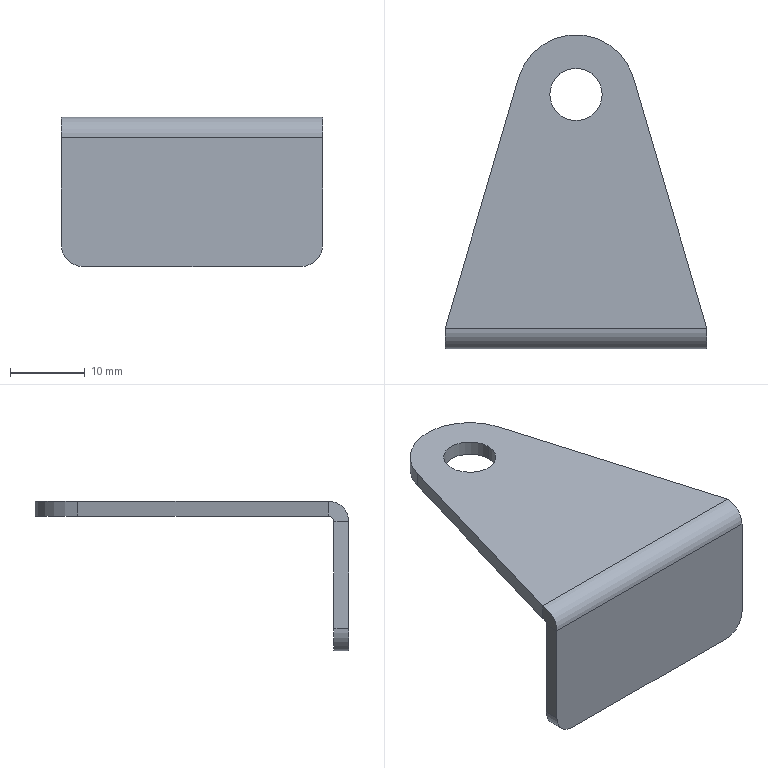Part | SolidWorks | features ICE 2, EdgeFlange 1, Fillet 1, FlatPattern 1, HoleWzd 1, SMBaseFlange 1, SheetMetal 1 | 1 solid | 18 faces | box 35 x 42 x 20 mm | volume 3132 mm3 | plane 11 | cylinder 7 | commonest cylinder face diameters 6 x2 7 x2 1.473 x1 5.473 x1 16 x1
STEP:
#1=CARTESIAN_POINT('',(3.5,32.,8.));
#2=VERTEX_POINT('',#1);
#3=CARTESIAN_POINT('',(-3.5,32.,8.));
#4=VERTEX_POINT('',#3);
#5=CARTESIAN_POINT('',(0.,32.,8.));
#6=DIRECTION('',(0.,0.,-1.));
#7=DIRECTION('',(-1.,0.,0.));
#8=AXIS2_PLACEMENT_3D('',#5,#6,#7);
#9=CIRCLE('',#8,3.5);
#10=EDGE_CURVE('',#2,#4,#9,.T.);
#11=ORIENTED_EDGE('',*,*,#10,.T.);
#12=CARTESIAN_POINT('',(-3.5,32.,10.));
#13=VERTEX_POINT('',#12);
#14=CARTESIAN_POINT('',(-3.5,32.,10.));
#15=DIRECTION('',(0.,0.,1.));
#16=VECTOR('',#15,1000.);
#17=LINE('',#14,#16);
#18=EDGE_CURVE('',#4,#13,#17,.T.);
#19=ORIENTED_EDGE('',*,*,#18,.T.);
#20=CARTESIAN_POINT('',(3.5,32.,10.));
#21=VERTEX_POINT('',#20);
#22=CARTESIAN_POINT('',(0.,32.,10.));
#23=DIRECTION('',(0.,0.,1.));
#24=DIRECTION('',(1.,0.,0.));
#25=AXIS2_PLACEMENT_3D('',#22,#23,#24);
#26=CIRCLE('',#25,3.5);
#27=EDGE_CURVE('',#13,#21,#26,.T.);
#28=ORIENTED_EDGE('',*,*,#27,.T.);
#29=CARTESIAN_POINT('',(3.5,32.,10.));
#30=DIRECTION('',(0.,0.,1.));
#31=VECTOR('',#30,1000.);
#32=LINE('',#29,#31);
#33=EDGE_CURVE('',#2,#21,#32,.T.);
#34=ORIENTED_EDGE('',*,*,#33,.F.);
#35=EDGE_LOOP('',(#11,#19,#28,#34));
#36=FACE_OUTER_BOUND('',#35,.T.);
#37=CARTESIAN_POINT('',(0.,32.,10.));
#38=DIRECTION('',(0.,0.,1.));
#39=DIRECTION('',(1.,0.,0.));
#40=AXIS2_PLACEMENT_3D('',#37,#38,#39);
#41=CYLINDRICAL_SURFACE('',#40,3.5);
#42=ADVANCED_FACE('',(#36),#41,.F.);
#43=CARTESIAN_POINT('',(0.,32.,10.));
#44=DIRECTION('',(0.,0.,1.));
#45=DIRECTION('',(1.,0.,0.));
#46=AXIS2_PLACEMENT_3D('',#43,#44,#45);
#47=CIRCLE('',#46,3.5);
#48=EDGE_CURVE('',#21,#13,#47,.T.);
#49=ORIENTED_EDGE('',*,*,#48,.F.);
#50=ORIENTED_EDGE('',*,*,#27,.F.);
#51=EDGE_LOOP('',(#49,#50));
#52=FACE_BOUND('',#51,.T.);
#53=CARTESIAN_POINT('',(-7.677,34.25,10.));
#54=VERTEX_POINT('',#53);
#55=CARTESIAN_POINT('',(7.677,34.25,10.));
#56=VERTEX_POINT('',#55);
#57=CARTESIAN_POINT('',(0.,32.,10.));
#58=DIRECTION('',(0.,0.,-1.));
#59=DIRECTION('',(-1.,0.,0.));
#60=AXIS2_PLACEMENT_3D('',#57,#58,#59);
#61=CIRCLE('',#60,8.);
#62=EDGE_CURVE('',#54,#56,#61,.T.);
#63=ORIENTED_EDGE('',*,*,#62,.F.);
#64=CARTESIAN_POINT('',(-17.5,0.7366,10.));
#65=VERTEX_POINT('',#64);
#66=CARTESIAN_POINT('',(-16.314,4.782,10.));
#67=DIRECTION('',(0.2813,0.9596,0.));
#68=VECTOR('',#67,1000.);
#69=LINE('',#66,#68);
#70=EDGE_CURVE('',#65,#54,#69,.T.);
#71=ORIENTED_EDGE('',*,*,#70,.F.);
#72=CARTESIAN_POINT('',(17.5,0.7366,10.));
#73=VERTEX_POINT('',#72);
#74=CARTESIAN_POINT('',(-17.5,0.7366,10.));
#75=DIRECTION('',(-1.,0.,0.));
#76=VECTOR('',#75,1000.);
#77=LINE('',#74,#76);
#78=EDGE_CURVE('',#73,#65,#77,.T.);
#79=ORIENTED_EDGE('',*,*,#78,.F.);
#80=CARTESIAN_POINT('',(16.314,4.782,10.));
#81=DIRECTION('',(0.2813,-0.9596,0.));
#82=VECTOR('',#81,1000.);
#83=LINE('',#80,#82);
#84=EDGE_CURVE('',#56,#73,#83,.T.);
#85=ORIENTED_EDGE('',*,*,#84,.F.);
#86=EDGE_LOOP('',(#63,#71,#79,#85));
#87=FACE_OUTER_BOUND('',#86,.T.);
#88=CARTESIAN_POINT('',(0.,0.,10.));
#89=DIRECTION('',(0.,0.,-1.));
#90=DIRECTION('',(-1.,0.,0.));
#91=AXIS2_PLACEMENT_3D('',#88,#89,#90);
#92=PLANE('',#91);
#93=ADVANCED_FACE('',(#52,#87),#92,.F.);
#94=ORIENTED_EDGE('',*,*,#10,.F.);
#95=CARTESIAN_POINT('',(0.,32.,8.));
#96=DIRECTION('',(0.,0.,-1.));
#97=DIRECTION('',(-1.,0.,0.));
#98=AXIS2_PLACEMENT_3D('',#95,#96,#97);
#99=CIRCLE('',#98,3.5);
#100=EDGE_CURVE('',#4,#2,#99,.T.);
#101=ORIENTED_EDGE('',*,*,#100,.F.);
#102=EDGE_LOOP('',(#94,#101));
#103=FACE_BOUND('',#102,.T.);
#104=CARTESIAN_POINT('',(-17.5,0.7366,8.));
#105=VERTEX_POINT('',#104);
#106=CARTESIAN_POINT('',(-7.677,34.25,8.));
#107=VERTEX_POINT('',#106);
#108=CARTESIAN_POINT('',(-16.314,4.782,8.));
#109=DIRECTION('',(0.2813,0.9596,0.));
#110=VECTOR('',#109,1000.);
#111=LINE('',#108,#110);
#112=EDGE_CURVE('',#105,#107,#111,.T.);
#113=ORIENTED_EDGE('',*,*,#112,.T.);
#114=CARTESIAN_POINT('',(7.677,34.25,8.));
#115=VERTEX_POINT('',#114);
#116=CARTESIAN_POINT('',(0.,32.,8.));
#117=DIRECTION('',(0.,0.,-1.));
#118=DIRECTION('',(-1.,0.,0.));
#119=AXIS2_PLACEMENT_3D('',#116,#117,#118);
#120=CIRCLE('',#119,8.);
#121=EDGE_CURVE('',#107,#115,#120,.T.);
#122=ORIENTED_EDGE('',*,*,#121,.T.);
#123=CARTESIAN_POINT('',(17.5,0.7366,8.));
#124=VERTEX_POINT('',#123);
#125=CARTESIAN_POINT('',(16.314,4.782,8.));
#126=DIRECTION('',(0.2813,-0.9596,0.));
#127=VECTOR('',#126,1000.);
#128=LINE('',#125,#127);
#129=EDGE_CURVE('',#115,#124,#128,.T.);
#130=ORIENTED_EDGE('',*,*,#129,.T.);
#131=CARTESIAN_POINT('',(-17.5,0.7366,8.));
#132=DIRECTION('',(1.,0.,0.));
#133=VECTOR('',#132,1000.);
#134=LINE('',#131,#133);
#135=EDGE_CURVE('',#105,#124,#134,.T.);
#136=ORIENTED_EDGE('',*,*,#135,.F.);
#137=EDGE_LOOP('',(#113,#122,#130,#136));
#138=FACE_OUTER_BOUND('',#137,.T.);
#139=CARTESIAN_POINT('',(0.,0.,8.));
#140=DIRECTION('',(0.,0.,-1.));
#141=DIRECTION('',(-1.,0.,0.));
#142=AXIS2_PLACEMENT_3D('',#139,#140,#141);
#143=PLANE('',#142);
#144=ADVANCED_FACE('',(#103,#138),#143,.T.);
#145=CARTESIAN_POINT('',(17.5,-2.,7.263));
#146=VERTEX_POINT('',#145);
#147=CARTESIAN_POINT('',(17.5,-2.,-7.));
#148=VERTEX_POINT('',#147);
#149=CARTESIAN_POINT('',(17.5,-2.,10.));
#150=DIRECTION('',(0.,0.,-1.));
#151=VECTOR('',#150,1000.);
#152=LINE('',#149,#151);
#153=EDGE_CURVE('',#146,#148,#152,.T.);
#154=ORIENTED_EDGE('',*,*,#153,.T.);
#155=CARTESIAN_POINT('',(17.5,0.,-7.));
#156=VERTEX_POINT('',#155);
#157=CARTESIAN_POINT('',(17.5,-2.,-7.));
#158=DIRECTION('',(0.,1.,0.));
#159=VECTOR('',#158,1000.);
#160=LINE('',#157,#159);
#161=EDGE_CURVE('',#148,#156,#160,.T.);
#162=ORIENTED_EDGE('',*,*,#161,.T.);
#163=CARTESIAN_POINT('',(17.5,0.,7.263));
#164=VERTEX_POINT('',#163);
#165=CARTESIAN_POINT('',(17.5,0.,10.));
#166=DIRECTION('',(0.,0.,-1.));
#167=VECTOR('',#166,1000.);
#168=LINE('',#165,#167);
#169=EDGE_CURVE('',#164,#156,#168,.T.);
#170=ORIENTED_EDGE('',*,*,#169,.F.);
#171=CARTESIAN_POINT('',(17.5,0.,7.263));
#172=DIRECTION('',(0.,-1.,0.));
#173=VECTOR('',#172,1000.);
#174=LINE('',#171,#173);
#175=EDGE_CURVE('',#164,#146,#174,.T.);
#176=ORIENTED_EDGE('',*,*,#175,.T.);
#177=EDGE_LOOP('',(#154,#162,#170,#176));
#178=FACE_OUTER_BOUND('',#177,.T.);
#179=CARTESIAN_POINT('',(17.5,-2.,10.));
#180=DIRECTION('',(1.,0.,0.));
#181=DIRECTION('',(0.,0.,-1.));
#182=AXIS2_PLACEMENT_3D('',#179,#180,#181);
#183=PLANE('',#182);
#184=ADVANCED_FACE('',(#178),#183,.T.);
#185=CARTESIAN_POINT('',(14.5,-2.,-10.));
#186=VERTEX_POINT('',#185);
#187=CARTESIAN_POINT('',(-14.5,-2.,-10.));
#188=VERTEX_POINT('',#187);
#189=CARTESIAN_POINT('',(-17.5,-2.,-10.));
#190=DIRECTION('',(-1.,0.,0.));
#191=VECTOR('',#190,1000.);
#192=LINE('',#189,#191);
#193=EDGE_CURVE('',#186,#188,#192,.T.);
#194=ORIENTED_EDGE('',*,*,#193,.F.);
#195=CARTESIAN_POINT('',(14.5,-2.,-7.));
#196=DIRECTION('',(0.,-1.,0.));
#197=DIRECTION('',(0.,0.,-1.));
#198=AXIS2_PLACEMENT_3D('',#195,#196,#197);
#199=CIRCLE('',#198,3.);
#200=EDGE_CURVE('',#186,#148,#199,.T.);
#201=ORIENTED_EDGE('',*,*,#200,.T.);
#202=ORIENTED_EDGE('',*,*,#153,.F.);
#203=CARTESIAN_POINT('',(-17.5,-2.,7.263));
#204=VERTEX_POINT('',#203);
#205=CARTESIAN_POINT('',(17.5,-2.,7.263));
#206=DIRECTION('',(-1.,0.,0.));
#207=VECTOR('',#206,1000.);
#208=LINE('',#205,#207);
#209=EDGE_CURVE('',#146,#204,#208,.T.);
#210=ORIENTED_EDGE('',*,*,#209,.T.);
#211=CARTESIAN_POINT('',(-17.5,-2.,-7.));
#212=VERTEX_POINT('',#211);
#213=CARTESIAN_POINT('',(-17.5,-2.,10.));
#214=DIRECTION('',(0.,0.,1.));
#215=VECTOR('',#214,1000.);
#216=LINE('',#213,#215);
#217=EDGE_CURVE('',#212,#204,#216,.T.);
#218=ORIENTED_EDGE('',*,*,#217,.F.);
#219=CARTESIAN_POINT('',(-14.5,-2.,-7.));
#220=DIRECTION('',(0.,-1.,0.));
#221=DIRECTION('',(0.,0.,-1.));
#222=AXIS2_PLACEMENT_3D('',#219,#220,#221);
#223=CIRCLE('',#222,3.);
#224=EDGE_CURVE('',#212,#188,#223,.T.);
#225=ORIENTED_EDGE('',*,*,#224,.T.);
#226=EDGE_LOOP('',(#194,#201,#202,#210,#218,#225));
#227=FACE_OUTER_BOUND('',#226,.T.);
#228=CARTESIAN_POINT('',(0.,-2.,0.));
#229=DIRECTION('',(0.,-1.,0.));
#230=DIRECTION('',(0.,0.,-1.));
#231=AXIS2_PLACEMENT_3D('',#228,#229,#230);
#232=PLANE('',#231);
#233=ADVANCED_FACE('',(#227),#232,.T.);
#234=ORIENTED_EDGE('',*,*,#169,.T.);
#235=CARTESIAN_POINT('',(14.5,0.,-10.));
#236=VERTEX_POINT('',#235);
#237=CARTESIAN_POINT('',(14.5,0.,-7.));
#238=DIRECTION('',(0.,1.,0.));
#239=DIRECTION('',(0.,0.,-1.));
#240=AXIS2_PLACEMENT_3D('',#237,#238,#239);
#241=CIRCLE('',#240,3.);
#242=EDGE_CURVE('',#156,#236,#241,.T.);
#243=ORIENTED_EDGE('',*,*,#242,.T.);
#244=CARTESIAN_POINT('',(-14.5,0.,-10.));
#245=VERTEX_POINT('',#244);
#246=CARTESIAN_POINT('',(-17.5,0.,-10.));
#247=DIRECTION('',(-1.,0.,0.));
#248=VECTOR('',#247,1000.);
#249=LINE('',#246,#248);
#250=EDGE_CURVE('',#236,#245,#249,.T.);
#251=ORIENTED_EDGE('',*,*,#250,.T.);
#252=CARTESIAN_POINT('',(-17.5,0.,-7.));
#253=VERTEX_POINT('',#252);
#254=CARTESIAN_POINT('',(-14.5,0.,-7.));
#255=DIRECTION('',(0.,1.,0.));
#256=DIRECTION('',(0.,0.,-1.));
#257=AXIS2_PLACEMENT_3D('',#254,#255,#256);
#258=CIRCLE('',#257,3.);
#259=EDGE_CURVE('',#245,#253,#258,.T.);
#260=ORIENTED_EDGE('',*,*,#259,.T.);
#261=CARTESIAN_POINT('',(-17.5,0.,7.263));
#262=VERTEX_POINT('',#261);
#263=CARTESIAN_POINT('',(-17.5,0.,10.));
#264=DIRECTION('',(0.,0.,1.));
#265=VECTOR('',#264,1000.);
#266=LINE('',#263,#265);
#267=EDGE_CURVE('',#253,#262,#266,.T.);
#268=ORIENTED_EDGE('',*,*,#267,.T.);
#269=CARTESIAN_POINT('',(17.5,0.,7.263));
#270=DIRECTION('',(-1.,0.,0.));
#271=VECTOR('',#270,1000.);
#272=LINE('',#269,#271);
#273=EDGE_CURVE('',#164,#262,#272,.T.);
#274=ORIENTED_EDGE('',*,*,#273,.F.);
#275=EDGE_LOOP('',(#234,#243,#251,#260,#268,#274));
#276=FACE_OUTER_BOUND('',#275,.T.);
#277=CARTESIAN_POINT('',(0.,0.,0.));
#278=DIRECTION('',(0.,-1.,0.));
#279=DIRECTION('',(0.,0.,-1.));
#280=AXIS2_PLACEMENT_3D('',#277,#278,#279);
#281=PLANE('',#280);
#282=ADVANCED_FACE('',(#276),#281,.F.);
#283=ORIENTED_EDGE('',*,*,#267,.F.);
#284=CARTESIAN_POINT('',(-17.5,-2.,-7.));
#285=DIRECTION('',(0.,-1.,0.));
#286=VECTOR('',#285,1000.);
#287=LINE('',#284,#286);
#288=EDGE_CURVE('',#253,#212,#287,.T.);
#289=ORIENTED_EDGE('',*,*,#288,.T.);
#290=ORIENTED_EDGE('',*,*,#217,.T.);
#291=CARTESIAN_POINT('',(-17.5,0.,7.263));
#292=DIRECTION('',(0.,-1.,0.));
#293=VECTOR('',#292,1000.);
#294=LINE('',#291,#293);
#295=EDGE_CURVE('',#262,#204,#294,.T.);
#296=ORIENTED_EDGE('',*,*,#295,.F.);
#297=EDGE_LOOP('',(#283,#289,#290,#296));
#298=FACE_OUTER_BOUND('',#297,.T.);
#299=CARTESIAN_POINT('',(-17.5,-2.,10.));
#300=DIRECTION('',(-1.,0.,0.));
#301=DIRECTION('',(0.,0.,1.));
#302=AXIS2_PLACEMENT_3D('',#299,#300,#301);
#303=PLANE('',#302);
#304=ADVANCED_FACE('',(#298),#303,.T.);
#305=ORIENTED_EDGE('',*,*,#250,.F.);
#306=CARTESIAN_POINT('',(14.5,-2.,-10.));
#307=DIRECTION('',(0.,-1.,0.));
#308=VECTOR('',#307,1000.);
#309=LINE('',#306,#308);
#310=EDGE_CURVE('',#236,#186,#309,.T.);
#311=ORIENTED_EDGE('',*,*,#310,.T.);
#312=ORIENTED_EDGE('',*,*,#193,.T.);
#313=CARTESIAN_POINT('',(-14.5,-2.,-10.));
#314=DIRECTION('',(0.,1.,0.));
#315=VECTOR('',#314,1000.);
#316=LINE('',#313,#315);
#317=EDGE_CURVE('',#188,#245,#316,.T.);
#318=ORIENTED_EDGE('',*,*,#317,.T.);
#319=EDGE_LOOP('',(#305,#311,#312,#318));
#320=FACE_OUTER_BOUND('',#319,.T.);
#321=CARTESIAN_POINT('',(-17.5,-2.,-10.));
#322=DIRECTION('',(0.,0.,-1.));
#323=DIRECTION('',(-1.,0.,0.));
#324=AXIS2_PLACEMENT_3D('',#321,#322,#323);
#325=PLANE('',#324);
#326=ADVANCED_FACE('',(#320),#325,.T.);
#327=CARTESIAN_POINT('',(-17.5,0.7366,10.));
#328=DIRECTION('',(0.,0.,1.));
#329=VECTOR('',#328,1000.);
#330=LINE('',#327,#329);
#331=EDGE_CURVE('',#105,#65,#330,.T.);
#332=ORIENTED_EDGE('',*,*,#331,.F.);
#333=CARTESIAN_POINT('',(-17.5,0.7366,7.263));
#334=DIRECTION('',(-1.,0.,0.));
#335=DIRECTION('',(0.,0.,-1.));
#336=AXIS2_PLACEMENT_3D('',#333,#334,#335);
#337=CIRCLE('',#336,0.7366);
#338=EDGE_CURVE('',#262,#105,#337,.T.);
#339=ORIENTED_EDGE('',*,*,#338,.F.);
#340=ORIENTED_EDGE('',*,*,#295,.T.);
#341=CARTESIAN_POINT('',(-17.5,0.7366,7.263));
#342=DIRECTION('',(-1.,0.,0.));
#343=DIRECTION('',(0.,0.,-1.));
#344=AXIS2_PLACEMENT_3D('',#341,#342,#343);
#345=CIRCLE('',#344,2.737);
#346=EDGE_CURVE('',#204,#65,#345,.T.);
#347=ORIENTED_EDGE('',*,*,#346,.T.);
#348=EDGE_LOOP('',(#332,#339,#340,#347));
#349=FACE_OUTER_BOUND('',#348,.T.);
#350=CARTESIAN_POINT('',(-17.5,0.7366,7.263));
#351=DIRECTION('',(-1.,0.,0.));
#352=DIRECTION('',(0.,0.,1.));
#353=AXIS2_PLACEMENT_3D('',#350,#351,#352);
#354=PLANE('',#353);
#355=ADVANCED_FACE('',(#349),#354,.T.);
#356=CARTESIAN_POINT('',(17.5,0.7366,7.263));
#357=DIRECTION('',(1.,0.,0.));
#358=DIRECTION('',(0.,0.,-1.));
#359=AXIS2_PLACEMENT_3D('',#356,#357,#358);
#360=CIRCLE('',#359,0.7366);
#361=EDGE_CURVE('',#124,#164,#360,.T.);
#362=ORIENTED_EDGE('',*,*,#361,.F.);
#363=CARTESIAN_POINT('',(17.5,0.7366,8.));
#364=DIRECTION('',(0.,0.,1.));
#365=VECTOR('',#364,1000.);
#366=LINE('',#363,#365);
#367=EDGE_CURVE('',#124,#73,#366,.T.);
#368=ORIENTED_EDGE('',*,*,#367,.T.);
#369=CARTESIAN_POINT('',(17.5,0.7366,7.263));
#370=DIRECTION('',(1.,0.,0.));
#371=DIRECTION('',(0.,0.,-1.));
#372=AXIS2_PLACEMENT_3D('',#369,#370,#371);
#373=CIRCLE('',#372,2.737);
#374=EDGE_CURVE('',#73,#146,#373,.T.);
#375=ORIENTED_EDGE('',*,*,#374,.T.);
#376=ORIENTED_EDGE('',*,*,#175,.F.);
#377=EDGE_LOOP('',(#362,#368,#375,#376));
#378=FACE_OUTER_BOUND('',#377,.T.);
#379=CARTESIAN_POINT('',(17.5,0.7366,7.263));
#380=DIRECTION('',(-1.,0.,0.));
#381=DIRECTION('',(0.,0.,1.));
#382=AXIS2_PLACEMENT_3D('',#379,#380,#381);
#383=PLANE('',#382);
#384=ADVANCED_FACE('',(#378),#383,.F.);
#385=ORIENTED_EDGE('',*,*,#209,.F.);
#386=ORIENTED_EDGE('',*,*,#374,.F.);
#387=ORIENTED_EDGE('',*,*,#78,.T.);
#388=ORIENTED_EDGE('',*,*,#346,.F.);
#389=EDGE_LOOP('',(#385,#386,#387,#388));
#390=FACE_OUTER_BOUND('',#389,.T.);
#391=CARTESIAN_POINT('',(17.5,0.7366,7.263));
#392=DIRECTION('',(1.,0.,0.));
#393=DIRECTION('',(0.,0.,1.));
#394=AXIS2_PLACEMENT_3D('',#391,#392,#393);
#395=CYLINDRICAL_SURFACE('',#394,2.737);
#396=ADVANCED_FACE('',(#390),#395,.T.);
#397=ORIENTED_EDGE('',*,*,#273,.T.);
#398=ORIENTED_EDGE('',*,*,#338,.T.);
#399=ORIENTED_EDGE('',*,*,#135,.T.);
#400=ORIENTED_EDGE('',*,*,#361,.T.);
#401=EDGE_LOOP('',(#397,#398,#399,#400));
#402=FACE_OUTER_BOUND('',#401,.T.);
#403=CARTESIAN_POINT('',(17.5,0.7366,7.263));
#404=DIRECTION('',(1.,0.,0.));
#405=DIRECTION('',(0.,0.,1.));
#406=AXIS2_PLACEMENT_3D('',#403,#404,#405);
#407=CYLINDRICAL_SURFACE('',#406,0.7366);
#408=ADVANCED_FACE('',(#402),#407,.F.);
#409=ORIENTED_EDGE('',*,*,#367,.F.);
#410=ORIENTED_EDGE('',*,*,#129,.F.);
#411=CARTESIAN_POINT('',(7.677,34.25,8.));
#412=DIRECTION('',(0.,0.,1.));
#413=VECTOR('',#412,1000.);
#414=LINE('',#411,#413);
#415=EDGE_CURVE('',#115,#56,#414,.T.);
#416=ORIENTED_EDGE('',*,*,#415,.T.);
#417=ORIENTED_EDGE('',*,*,#84,.T.);
#418=EDGE_LOOP('',(#409,#410,#416,#417));
#419=FACE_OUTER_BOUND('',#418,.T.);
#420=CARTESIAN_POINT('',(16.314,4.782,8.));
#421=DIRECTION('',(0.9596,0.2813,0.));
#422=DIRECTION('',(0.2813,-0.9596,0.));
#423=AXIS2_PLACEMENT_3D('',#420,#421,#422);
#424=PLANE('',#423);
#425=ADVANCED_FACE('',(#419),#424,.T.);
#426=ORIENTED_EDGE('',*,*,#415,.F.);
#427=ORIENTED_EDGE('',*,*,#121,.F.);
#428=CARTESIAN_POINT('',(-7.677,34.25,8.));
#429=DIRECTION('',(0.,0.,1.));
#430=VECTOR('',#429,1000.);
#431=LINE('',#428,#430);
#432=EDGE_CURVE('',#107,#54,#431,.T.);
#433=ORIENTED_EDGE('',*,*,#432,.T.);
#434=ORIENTED_EDGE('',*,*,#62,.T.);
#435=EDGE_LOOP('',(#426,#427,#433,#434));
#436=FACE_OUTER_BOUND('',#435,.T.);
#437=CARTESIAN_POINT('',(0.,32.,8.));
#438=DIRECTION('',(0.,0.,-1.));
#439=DIRECTION('',(-1.,0.,0.));
#440=AXIS2_PLACEMENT_3D('',#437,#438,#439);
#441=CYLINDRICAL_SURFACE('',#440,8.);
#442=ADVANCED_FACE('',(#436),#441,.T.);
#443=ORIENTED_EDGE('',*,*,#432,.F.);
#444=ORIENTED_EDGE('',*,*,#112,.F.);
#445=ORIENTED_EDGE('',*,*,#331,.T.);
#446=ORIENTED_EDGE('',*,*,#70,.T.);
#447=EDGE_LOOP('',(#443,#444,#445,#446));
#448=FACE_OUTER_BOUND('',#447,.T.);
#449=CARTESIAN_POINT('',(-16.314,4.782,8.));
#450=DIRECTION('',(-0.9596,0.2813,0.));
#451=DIRECTION('',(0.2813,0.9596,0.));
#452=AXIS2_PLACEMENT_3D('',#449,#450,#451);
#453=PLANE('',#452);
#454=ADVANCED_FACE('',(#448),#453,.T.);
#455=ORIENTED_EDGE('',*,*,#18,.F.);
#456=ORIENTED_EDGE('',*,*,#100,.T.);
#457=ORIENTED_EDGE('',*,*,#33,.T.);
#458=ORIENTED_EDGE('',*,*,#48,.T.);
#459=EDGE_LOOP('',(#455,#456,#457,#458));
#460=FACE_OUTER_BOUND('',#459,.T.);
#461=CARTESIAN_POINT('',(0.,32.,10.));
#462=DIRECTION('',(0.,0.,1.));
#463=DIRECTION('',(1.,0.,0.));
#464=AXIS2_PLACEMENT_3D('',#461,#462,#463);
#465=CYLINDRICAL_SURFACE('',#464,3.5);
#466=ADVANCED_FACE('',(#460),#465,.F.);
#467=ORIENTED_EDGE('',*,*,#200,.F.);
#468=ORIENTED_EDGE('',*,*,#310,.F.);
#469=ORIENTED_EDGE('',*,*,#242,.F.);
#470=ORIENTED_EDGE('',*,*,#161,.F.);
#471=EDGE_LOOP('',(#467,#468,#469,#470));
#472=FACE_OUTER_BOUND('',#471,.T.);
#473=CARTESIAN_POINT('',(14.5,-2.,-7.));
#474=DIRECTION('',(0.,1.,0.));
#475=DIRECTION('',(0.,0.,1.));
#476=AXIS2_PLACEMENT_3D('',#473,#474,#475);
#477=CYLINDRICAL_SURFACE('',#476,3.);
#478=ADVANCED_FACE('',(#472),#477,.T.);
#479=ORIENTED_EDGE('',*,*,#224,.F.);
#480=ORIENTED_EDGE('',*,*,#288,.F.);
#481=ORIENTED_EDGE('',*,*,#259,.F.);
#482=ORIENTED_EDGE('',*,*,#317,.F.);
#483=EDGE_LOOP('',(#479,#480,#481,#482));
#484=FACE_OUTER_BOUND('',#483,.T.);
#485=CARTESIAN_POINT('',(-14.5,-2.,-7.));
#486=DIRECTION('',(0.,1.,0.));
#487=DIRECTION('',(0.,0.,1.));
#488=AXIS2_PLACEMENT_3D('',#485,#486,#487);
#489=CYLINDRICAL_SURFACE('',#488,3.);
#490=ADVANCED_FACE('',(#484),#489,.T.);
#491=CLOSED_SHELL('',(#42,#93,#144,#184,#233,#282,#304,#326,#355,#384,#396,#408,#425,#442,#454,#466,#478,#490));
#492=MANIFOLD_SOLID_BREP('',#491);
#493=CARTESIAN_POINT('',(0.,0.,0.));
#494=DIRECTION('',(0.,0.,1.));
#495=DIRECTION('',(1.,0.,0.));
#496=AXIS2_PLACEMENT_3D('',#493,#494,#495);
#497=(LENGTH_UNIT()NAMED_UNIT(*)SI_UNIT(.MILLI.,.METRE.));
#498=UNCERTAINTY_MEASURE_WITH_UNIT(LENGTH_MEASURE(0.00001),#497,'','');
#499=(NAMED_UNIT(*)PLANE_ANGLE_UNIT()SI_UNIT($,.RADIAN.));
#500=(NAMED_UNIT(*)SI_UNIT($,.STERADIAN.)SOLID_ANGLE_UNIT());
#501=(GEOMETRIC_REPRESENTATION_CONTEXT(3)GLOBAL_UNCERTAINTY_ASSIGNED_CONTEXT((#498))GLOBAL_UNIT_ASSIGNED_CONTEXT((#497,#499,#500))REPRESENTATION_CONTEXT('',''));
#502=ADVANCED_BREP_SHAPE_REPRESENTATION('',(#492,#496),#501);